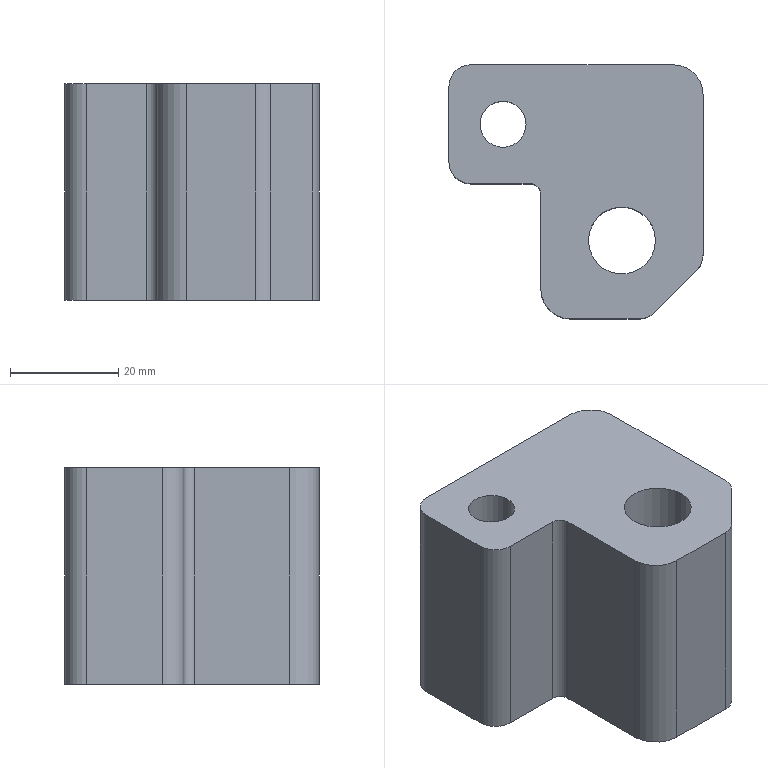Part | NX | features PS-8 2 | 1 solid | 20 faces | box 47 x 47 x 40 mm | volume 60211 mm3 | plane 10 | cylinder 10 | commonest cylinder face diameters 8 x4 11 x2 4 x1 8.5 x1 12.4 x1 14.5 x1
STEP:
#1=CARTESIAN_POINT('',(2465.297,-906.795,860.716));
#2=VERTEX_POINT('',#1);
#3=CARTESIAN_POINT('',(2459.097,-906.795,860.716));
#4=DIRECTION('',(0.,0.,1.));
#5=DIRECTION('',(1.,0.,0.));
#6=AXIS2_PLACEMENT_3D('',#3,#4,#5);
#7=CIRCLE('',#6,6.2);
#8=EDGE_CURVE('',#2,#2,#7,.T.);
#9=ORIENTED_EDGE('',*,*,#8,.T.);
#10=EDGE_LOOP('',(#9));
#11=FACE_BOUND('',#10,.T.);
#12=CARTESIAN_POINT('',(2444.347,-885.295,860.716));
#13=VERTEX_POINT('',#12);
#14=CARTESIAN_POINT('',(2437.097,-885.295,860.716));
#15=DIRECTION('',(0.,0.,1.));
#16=DIRECTION('',(1.,0.,0.));
#17=AXIS2_PLACEMENT_3D('',#14,#15,#16);
#18=CIRCLE('',#17,7.25);
#19=EDGE_CURVE('',#13,#13,#18,.T.);
#20=ORIENTED_EDGE('',*,*,#19,.T.);
#21=EDGE_LOOP('',(#20));
#22=FACE_BOUND('',#21,.T.);
#23=CARTESIAN_POINT('',(2444.097,-898.295,860.716));
#24=VERTEX_POINT('',#23);
#25=CARTESIAN_POINT('',(2444.097,-915.795,860.716));
#26=VERTEX_POINT('',#25);
#27=CARTESIAN_POINT('',(2444.097,0.,860.716));
#28=DIRECTION('',(0.,-1.,0.));
#29=VECTOR('',#28,1000.);
#30=LINE('',#27,#29);
#31=EDGE_CURVE('',#24,#26,#30,.T.);
#32=ORIENTED_EDGE('',*,*,#31,.F.);
#33=CARTESIAN_POINT('',(2442.097,-896.295,860.716));
#34=VERTEX_POINT('',#33);
#35=CARTESIAN_POINT('',(2442.097,-898.295,860.716));
#36=DIRECTION('',(0.,0.,1.));
#37=DIRECTION('',(1.,0.,0.));
#38=AXIS2_PLACEMENT_3D('',#35,#36,#37);
#39=CIRCLE('',#38,2.);
#40=EDGE_CURVE('',#24,#34,#39,.T.);
#41=ORIENTED_EDGE('',*,*,#40,.T.);
#42=CARTESIAN_POINT('',(2431.097,-896.295,860.716));
#43=VERTEX_POINT('',#42);
#44=CARTESIAN_POINT('',(2437.597,-896.295,860.716));
#45=DIRECTION('',(1.,0.,0.));
#46=VECTOR('',#45,1000.);
#47=LINE('',#44,#46);
#48=EDGE_CURVE('',#43,#34,#47,.T.);
#49=ORIENTED_EDGE('',*,*,#48,.F.);
#50=CARTESIAN_POINT('',(2427.097,-892.295,860.716));
#51=VERTEX_POINT('',#50);
#52=CARTESIAN_POINT('',(2431.097,-892.295,860.716));
#53=DIRECTION('',(0.,0.,1.));
#54=DIRECTION('',(1.,0.,0.));
#55=AXIS2_PLACEMENT_3D('',#52,#53,#54);
#56=CIRCLE('',#55,4.);
#57=EDGE_CURVE('',#43,#51,#56,.F.);
#58=ORIENTED_EDGE('',*,*,#57,.T.);
#59=CARTESIAN_POINT('',(2427.097,-878.295,860.716));
#60=VERTEX_POINT('',#59);
#61=CARTESIAN_POINT('',(2427.097,0.,860.716));
#62=DIRECTION('',(0.,-1.,0.));
#63=VECTOR('',#62,1000.);
#64=LINE('',#61,#63);
#65=EDGE_CURVE('',#60,#51,#64,.T.);
#66=ORIENTED_EDGE('',*,*,#65,.F.);
#67=CARTESIAN_POINT('',(2431.097,-874.295,860.716));
#68=VERTEX_POINT('',#67);
#69=CARTESIAN_POINT('',(2431.097,-878.295,860.716));
#70=DIRECTION('',(0.,0.,1.));
#71=DIRECTION('',(1.,0.,0.));
#72=AXIS2_PLACEMENT_3D('',#69,#70,#71);
#73=CIRCLE('',#72,4.);
#74=EDGE_CURVE('',#60,#68,#73,.F.);
#75=ORIENTED_EDGE('',*,*,#74,.T.);
#76=CARTESIAN_POINT('',(2468.597,-874.295,860.716));
#77=VERTEX_POINT('',#76);
#78=CARTESIAN_POINT('',(2468.597,-874.295,860.716));
#79=DIRECTION('',(1.,0.,0.));
#80=VECTOR('',#79,1000.);
#81=LINE('',#78,#80);
#82=EDGE_CURVE('',#68,#77,#81,.T.);
#83=ORIENTED_EDGE('',*,*,#82,.T.);
#84=CARTESIAN_POINT('',(2474.097,-879.795,860.716));
#85=VERTEX_POINT('',#84);
#86=CARTESIAN_POINT('',(2468.597,-879.795,860.716));
#87=DIRECTION('',(0.,0.,1.));
#88=DIRECTION('',(1.,0.,0.));
#89=AXIS2_PLACEMENT_3D('',#86,#87,#88);
#90=CIRCLE('',#89,5.5);
#91=EDGE_CURVE('',#85,#77,#90,.T.);
#92=ORIENTED_EDGE('',*,*,#91,.F.);
#93=CARTESIAN_POINT('',(2474.097,-909.467,860.716));
#94=VERTEX_POINT('',#93);
#95=CARTESIAN_POINT('',(2474.097,0.,860.716));
#96=DIRECTION('',(0.,1.,0.));
#97=VECTOR('',#96,1000.);
#98=LINE('',#95,#97);
#99=EDGE_CURVE('',#94,#85,#98,.T.);
#100=ORIENTED_EDGE('',*,*,#99,.F.);
#101=CARTESIAN_POINT('',(2472.926,-912.295,860.716));
#102=VERTEX_POINT('',#101);
#103=CARTESIAN_POINT('',(2470.097,-909.467,860.716));
#104=DIRECTION('',(0.,0.,1.));
#105=DIRECTION('',(1.,0.,0.));
#106=AXIS2_PLACEMENT_3D('',#103,#104,#105);
#107=CIRCLE('',#106,4.);
#108=EDGE_CURVE('',#94,#102,#107,.F.);
#109=ORIENTED_EDGE('',*,*,#108,.T.);
#110=CARTESIAN_POINT('',(2465.097,-920.124,860.716));
#111=VERTEX_POINT('',#110);
#112=CARTESIAN_POINT('',(1692.61,-1692.61,860.716));
#113=DIRECTION('',(0.7071,0.7071,0.));
#114=VECTOR('',#113,1000.);
#115=LINE('',#112,#114);
#116=EDGE_CURVE('',#111,#102,#115,.T.);
#117=ORIENTED_EDGE('',*,*,#116,.F.);
#118=CARTESIAN_POINT('',(2462.269,-921.295,860.716));
#119=VERTEX_POINT('',#118);
#120=CARTESIAN_POINT('',(2462.269,-917.295,860.716));
#121=DIRECTION('',(0.,0.,1.));
#122=DIRECTION('',(1.,0.,0.));
#123=AXIS2_PLACEMENT_3D('',#120,#121,#122);
#124=CIRCLE('',#123,4.);
#125=EDGE_CURVE('',#119,#111,#124,.T.);
#126=ORIENTED_EDGE('',*,*,#125,.F.);
#127=CARTESIAN_POINT('',(2449.597,-921.295,860.716));
#128=VERTEX_POINT('',#127);
#129=CARTESIAN_POINT('',(2449.597,-921.295,860.716));
#130=DIRECTION('',(-1.,0.,0.));
#131=VECTOR('',#130,1000.);
#132=LINE('',#129,#131);
#133=EDGE_CURVE('',#119,#128,#132,.T.);
#134=ORIENTED_EDGE('',*,*,#133,.T.);
#135=CARTESIAN_POINT('',(2449.597,-915.795,860.716));
#136=DIRECTION('',(0.,0.,1.));
#137=DIRECTION('',(1.,0.,0.));
#138=AXIS2_PLACEMENT_3D('',#135,#136,#137);
#139=CIRCLE('',#138,5.5);
#140=EDGE_CURVE('',#128,#26,#139,.F.);
#141=ORIENTED_EDGE('',*,*,#140,.T.);
#142=EDGE_LOOP('',(#32,#41,#49,#58,#66,#75,#83,#92,#100,#109,#117,#126,#134,#141));
#143=FACE_BOUND('',#142,.T.);
#144=CARTESIAN_POINT('',(0.,0.,860.716));
#145=DIRECTION('',(0.,0.,1.));
#146=DIRECTION('',(1.,0.,0.));
#147=AXIS2_PLACEMENT_3D('',#144,#145,#146);
#148=PLANE('',#147);
#149=ADVANCED_FACE('',(#11,#22,#143),#148,.F.);
#150=CARTESIAN_POINT('',(2444.097,-898.295,900.716));
#151=VERTEX_POINT('',#150);
#152=CARTESIAN_POINT('',(2444.097,-915.795,900.716));
#153=VERTEX_POINT('',#152);
#154=CARTESIAN_POINT('',(2444.097,0.,900.716));
#155=DIRECTION('',(0.,-1.,0.));
#156=VECTOR('',#155,1000.);
#157=LINE('',#154,#156);
#158=EDGE_CURVE('',#151,#153,#157,.T.);
#159=ORIENTED_EDGE('',*,*,#158,.F.);
#160=CARTESIAN_POINT('',(2444.097,-898.295,830.716));
#161=DIRECTION('',(0.,0.,1.));
#162=VECTOR('',#161,1000.);
#163=LINE('',#160,#162);
#164=EDGE_CURVE('',#151,#24,#163,.F.);
#165=ORIENTED_EDGE('',*,*,#164,.T.);
#166=ORIENTED_EDGE('',*,*,#31,.T.);
#167=CARTESIAN_POINT('',(2444.097,-915.795,830.716));
#168=DIRECTION('',(0.,0.,1.));
#169=VECTOR('',#168,1000.);
#170=LINE('',#167,#169);
#171=EDGE_CURVE('',#153,#26,#170,.F.);
#172=ORIENTED_EDGE('',*,*,#171,.F.);
#173=EDGE_LOOP('',(#159,#165,#166,#172));
#174=FACE_BOUND('',#173,.T.);
#175=CARTESIAN_POINT('',(2444.097,-881.795,830.716));
#176=DIRECTION('',(-1.,0.,0.));
#177=DIRECTION('',(0.,0.,1.));
#178=AXIS2_PLACEMENT_3D('',#175,#176,#177);
#179=PLANE('',#178);
#180=ADVANCED_FACE('',(#174),#179,.T.);
#181=ORIENTED_EDGE('',*,*,#171,.T.);
#182=ORIENTED_EDGE('',*,*,#140,.F.);
#183=CARTESIAN_POINT('',(2449.597,-921.295,900.716));
#184=VERTEX_POINT('',#183);
#185=CARTESIAN_POINT('',(2449.597,-921.295,830.716));
#186=DIRECTION('',(0.,0.,-1.));
#187=VECTOR('',#186,1000.);
#188=LINE('',#185,#187);
#189=EDGE_CURVE('',#184,#128,#188,.T.);
#190=ORIENTED_EDGE('',*,*,#189,.F.);
#191=CARTESIAN_POINT('',(2449.597,-915.795,900.716));
#192=DIRECTION('',(0.,0.,1.));
#193=DIRECTION('',(1.,0.,0.));
#194=AXIS2_PLACEMENT_3D('',#191,#192,#193);
#195=CIRCLE('',#194,5.5);
#196=EDGE_CURVE('',#184,#153,#195,.F.);
#197=ORIENTED_EDGE('',*,*,#196,.T.);
#198=EDGE_LOOP('',(#181,#182,#190,#197));
#199=FACE_BOUND('',#198,.T.);
#200=CARTESIAN_POINT('',(2449.597,-915.795,830.716));
#201=DIRECTION('',(0.,0.,1.));
#202=DIRECTION('',(1.,0.,0.));
#203=AXIS2_PLACEMENT_3D('',#200,#201,#202);
#204=CYLINDRICAL_SURFACE('',#203,5.5);
#205=ADVANCED_FACE('',(#199),#204,.T.);
#206=ORIENTED_EDGE('',*,*,#189,.T.);
#207=ORIENTED_EDGE('',*,*,#133,.F.);
#208=CARTESIAN_POINT('',(2462.269,-921.295,900.716));
#209=VERTEX_POINT('',#208);
#210=CARTESIAN_POINT('',(2462.269,-921.295,830.716));
#211=DIRECTION('',(0.,0.,1.));
#212=VECTOR('',#211,1000.);
#213=LINE('',#210,#212);
#214=EDGE_CURVE('',#209,#119,#213,.F.);
#215=ORIENTED_EDGE('',*,*,#214,.F.);
#216=CARTESIAN_POINT('',(0.,-921.295,900.716));
#217=DIRECTION('',(1.,0.,0.));
#218=VECTOR('',#217,1000.);
#219=LINE('',#216,#218);
#220=EDGE_CURVE('',#184,#209,#219,.T.);
#221=ORIENTED_EDGE('',*,*,#220,.F.);
#222=EDGE_LOOP('',(#206,#207,#215,#221));
#223=FACE_BOUND('',#222,.T.);
#224=CARTESIAN_POINT('',(2449.597,-921.295,830.716));
#225=DIRECTION('',(0.,-1.,0.));
#226=DIRECTION('',(0.,0.,-1.));
#227=AXIS2_PLACEMENT_3D('',#224,#225,#226);
#228=PLANE('',#227);
#229=ADVANCED_FACE('',(#223),#228,.T.);
#230=ORIENTED_EDGE('',*,*,#214,.T.);
#231=ORIENTED_EDGE('',*,*,#125,.T.);
#232=CARTESIAN_POINT('',(2465.097,-920.124,900.716));
#233=VERTEX_POINT('',#232);
#234=CARTESIAN_POINT('',(2465.097,-920.124,830.716));
#235=DIRECTION('',(0.,0.,1.));
#236=VECTOR('',#235,1000.);
#237=LINE('',#234,#236);
#238=EDGE_CURVE('',#233,#111,#237,.F.);
#239=ORIENTED_EDGE('',*,*,#238,.F.);
#240=CARTESIAN_POINT('',(2462.269,-917.295,900.716));
#241=DIRECTION('',(0.,0.,1.));
#242=DIRECTION('',(1.,0.,0.));
#243=AXIS2_PLACEMENT_3D('',#240,#241,#242);
#244=CIRCLE('',#243,4.);
#245=EDGE_CURVE('',#209,#233,#244,.T.);
#246=ORIENTED_EDGE('',*,*,#245,.F.);
#247=EDGE_LOOP('',(#230,#231,#239,#246));
#248=FACE_BOUND('',#247,.T.);
#249=CARTESIAN_POINT('',(2462.269,-917.295,830.716));
#250=DIRECTION('',(0.,0.,1.));
#251=DIRECTION('',(1.,0.,0.));
#252=AXIS2_PLACEMENT_3D('',#249,#250,#251);
#253=CYLINDRICAL_SURFACE('',#252,4.);
#254=ADVANCED_FACE('',(#248),#253,.T.);
#255=ORIENTED_EDGE('',*,*,#238,.T.);
#256=ORIENTED_EDGE('',*,*,#116,.T.);
#257=CARTESIAN_POINT('',(2472.926,-912.295,900.716));
#258=VERTEX_POINT('',#257);
#259=CARTESIAN_POINT('',(2472.926,-912.295,830.716));
#260=DIRECTION('',(0.,0.,1.));
#261=VECTOR('',#260,1000.);
#262=LINE('',#259,#261);
#263=EDGE_CURVE('',#258,#102,#262,.F.);
#264=ORIENTED_EDGE('',*,*,#263,.F.);
#265=CARTESIAN_POINT('',(1692.61,-1692.61,900.716));
#266=DIRECTION('',(0.7071,0.7071,0.));
#267=VECTOR('',#266,1000.);
#268=LINE('',#265,#267);
#269=EDGE_CURVE('',#233,#258,#268,.T.);
#270=ORIENTED_EDGE('',*,*,#269,.F.);
#271=EDGE_LOOP('',(#255,#256,#264,#270));
#272=FACE_BOUND('',#271,.T.);
#273=CARTESIAN_POINT('',(2465.097,-920.124,830.716));
#274=DIRECTION('',(0.7071,-0.7071,0.));
#275=DIRECTION('',(0.7071,0.7071,0.));
#276=AXIS2_PLACEMENT_3D('',#273,#274,#275);
#277=PLANE('',#276);
#278=ADVANCED_FACE('',(#272),#277,.T.);
#279=ORIENTED_EDGE('',*,*,#263,.T.);
#280=ORIENTED_EDGE('',*,*,#108,.F.);
#281=CARTESIAN_POINT('',(2474.097,-909.467,900.716));
#282=VERTEX_POINT('',#281);
#283=CARTESIAN_POINT('',(2474.097,-909.467,830.716));
#284=DIRECTION('',(0.,0.,-1.));
#285=VECTOR('',#284,1000.);
#286=LINE('',#283,#285);
#287=EDGE_CURVE('',#282,#94,#286,.T.);
#288=ORIENTED_EDGE('',*,*,#287,.F.);
#289=CARTESIAN_POINT('',(2470.097,-909.467,900.716));
#290=DIRECTION('',(0.,0.,1.));
#291=DIRECTION('',(1.,0.,0.));
#292=AXIS2_PLACEMENT_3D('',#289,#290,#291);
#293=CIRCLE('',#292,4.);
#294=EDGE_CURVE('',#282,#258,#293,.F.);
#295=ORIENTED_EDGE('',*,*,#294,.T.);
#296=EDGE_LOOP('',(#279,#280,#288,#295));
#297=FACE_BOUND('',#296,.T.);
#298=CARTESIAN_POINT('',(2470.097,-909.467,830.716));
#299=DIRECTION('',(0.,0.,1.));
#300=DIRECTION('',(1.,0.,0.));
#301=AXIS2_PLACEMENT_3D('',#298,#299,#300);
#302=CYLINDRICAL_SURFACE('',#301,4.);
#303=ADVANCED_FACE('',(#297),#302,.T.);
#304=ORIENTED_EDGE('',*,*,#287,.T.);
#305=ORIENTED_EDGE('',*,*,#99,.T.);
#306=CARTESIAN_POINT('',(2474.097,-879.795,900.716));
#307=VERTEX_POINT('',#306);
#308=CARTESIAN_POINT('',(2474.097,-879.795,830.716));
#309=DIRECTION('',(0.,0.,1.));
#310=VECTOR('',#309,1000.);
#311=LINE('',#308,#310);
#312=EDGE_CURVE('',#307,#85,#311,.F.);
#313=ORIENTED_EDGE('',*,*,#312,.F.);
#314=CARTESIAN_POINT('',(2474.097,-909.467,900.716));
#315=DIRECTION('',(0.,-1.,0.));
#316=VECTOR('',#315,1000.);
#317=LINE('',#314,#316);
#318=EDGE_CURVE('',#307,#282,#317,.T.);
#319=ORIENTED_EDGE('',*,*,#318,.T.);
#320=EDGE_LOOP('',(#304,#305,#313,#319));
#321=FACE_BOUND('',#320,.T.);
#322=CARTESIAN_POINT('',(2474.097,-909.467,830.716));
#323=DIRECTION('',(1.,0.,0.));
#324=DIRECTION('',(0.,0.,-1.));
#325=AXIS2_PLACEMENT_3D('',#322,#323,#324);
#326=PLANE('',#325);
#327=ADVANCED_FACE('',(#321),#326,.T.);
#328=ORIENTED_EDGE('',*,*,#312,.T.);
#329=ORIENTED_EDGE('',*,*,#91,.T.);
#330=CARTESIAN_POINT('',(2468.597,-874.295,900.716));
#331=VERTEX_POINT('',#330);
#332=CARTESIAN_POINT('',(2468.597,-874.295,830.716));
#333=DIRECTION('',(0.,0.,1.));
#334=VECTOR('',#333,1000.);
#335=LINE('',#332,#334);
#336=EDGE_CURVE('',#331,#77,#335,.F.);
#337=ORIENTED_EDGE('',*,*,#336,.F.);
#338=CARTESIAN_POINT('',(2468.597,-879.795,900.716));
#339=DIRECTION('',(0.,0.,1.));
#340=DIRECTION('',(1.,0.,0.));
#341=AXIS2_PLACEMENT_3D('',#338,#339,#340);
#342=CIRCLE('',#341,5.5);
#343=EDGE_CURVE('',#307,#331,#342,.T.);
#344=ORIENTED_EDGE('',*,*,#343,.F.);
#345=EDGE_LOOP('',(#328,#329,#337,#344));
#346=FACE_BOUND('',#345,.T.);
#347=CARTESIAN_POINT('',(2468.597,-879.795,830.716));
#348=DIRECTION('',(0.,0.,1.));
#349=DIRECTION('',(1.,0.,0.));
#350=AXIS2_PLACEMENT_3D('',#347,#348,#349);
#351=CYLINDRICAL_SURFACE('',#350,5.5);
#352=ADVANCED_FACE('',(#346),#351,.T.);
#353=ORIENTED_EDGE('',*,*,#82,.F.);
#354=CARTESIAN_POINT('',(2431.097,-874.295,900.716));
#355=VERTEX_POINT('',#354);
#356=CARTESIAN_POINT('',(2431.097,-874.295,830.716));
#357=DIRECTION('',(0.,0.,1.));
#358=VECTOR('',#357,1000.);
#359=LINE('',#356,#358);
#360=EDGE_CURVE('',#68,#355,#359,.T.);
#361=ORIENTED_EDGE('',*,*,#360,.T.);
#362=CARTESIAN_POINT('',(2468.597,-874.295,900.716));
#363=DIRECTION('',(1.,0.,0.));
#364=VECTOR('',#363,1000.);
#365=LINE('',#362,#364);
#366=EDGE_CURVE('',#355,#331,#365,.T.);
#367=ORIENTED_EDGE('',*,*,#366,.T.);
#368=ORIENTED_EDGE('',*,*,#336,.T.);
#369=EDGE_LOOP('',(#353,#361,#367,#368));
#370=FACE_BOUND('',#369,.T.);
#371=CARTESIAN_POINT('',(2468.597,-874.295,830.716));
#372=DIRECTION('',(0.,1.,0.));
#373=DIRECTION('',(0.,0.,1.));
#374=AXIS2_PLACEMENT_3D('',#371,#372,#373);
#375=PLANE('',#374);
#376=ADVANCED_FACE('',(#370),#375,.T.);
#377=ORIENTED_EDGE('',*,*,#65,.T.);
#378=CARTESIAN_POINT('',(2427.097,-892.295,900.716));
#379=VERTEX_POINT('',#378);
#380=CARTESIAN_POINT('',(2427.097,-892.295,830.716));
#381=DIRECTION('',(0.,0.,1.));
#382=VECTOR('',#381,1000.);
#383=LINE('',#380,#382);
#384=EDGE_CURVE('',#51,#379,#383,.T.);
#385=ORIENTED_EDGE('',*,*,#384,.T.);
#386=CARTESIAN_POINT('',(2427.097,-878.295,900.716));
#387=VERTEX_POINT('',#386);
#388=CARTESIAN_POINT('',(2427.097,-881.795,900.716));
#389=DIRECTION('',(0.,1.,0.));
#390=VECTOR('',#389,1000.);
#391=LINE('',#388,#390);
#392=EDGE_CURVE('',#379,#387,#391,.T.);
#393=ORIENTED_EDGE('',*,*,#392,.T.);
#394=CARTESIAN_POINT('',(2427.097,-878.295,830.716));
#395=DIRECTION('',(0.,0.,1.));
#396=VECTOR('',#395,1000.);
#397=LINE('',#394,#396);
#398=EDGE_CURVE('',#387,#60,#397,.F.);
#399=ORIENTED_EDGE('',*,*,#398,.T.);
#400=EDGE_LOOP('',(#377,#385,#393,#399));
#401=FACE_BOUND('',#400,.T.);
#402=CARTESIAN_POINT('',(2427.097,-881.795,830.716));
#403=DIRECTION('',(-1.,0.,0.));
#404=DIRECTION('',(0.,0.,1.));
#405=AXIS2_PLACEMENT_3D('',#402,#403,#404);
#406=PLANE('',#405);
#407=ADVANCED_FACE('',(#401),#406,.T.);
#408=ORIENTED_EDGE('',*,*,#48,.T.);
#409=CARTESIAN_POINT('',(2442.097,-896.295,900.716));
#410=VERTEX_POINT('',#409);
#411=CARTESIAN_POINT('',(2442.097,-896.295,875.716));
#412=DIRECTION('',(0.,0.,1.));
#413=VECTOR('',#412,1000.);
#414=LINE('',#411,#413);
#415=EDGE_CURVE('',#34,#410,#414,.T.);
#416=ORIENTED_EDGE('',*,*,#415,.T.);
#417=CARTESIAN_POINT('',(2431.097,-896.295,900.716));
#418=VERTEX_POINT('',#417);
#419=CARTESIAN_POINT('',(2437.597,-896.295,900.716));
#420=DIRECTION('',(1.,0.,0.));
#421=VECTOR('',#420,1000.);
#422=LINE('',#419,#421);
#423=EDGE_CURVE('',#418,#410,#422,.T.);
#424=ORIENTED_EDGE('',*,*,#423,.F.);
#425=CARTESIAN_POINT('',(2431.097,-896.295,875.716));
#426=DIRECTION('',(0.,0.,1.));
#427=VECTOR('',#426,1000.);
#428=LINE('',#425,#427);
#429=EDGE_CURVE('',#418,#43,#428,.F.);
#430=ORIENTED_EDGE('',*,*,#429,.T.);
#431=EDGE_LOOP('',(#408,#416,#424,#430));
#432=FACE_BOUND('',#431,.T.);
#433=CARTESIAN_POINT('',(2437.597,-896.295,875.716));
#434=DIRECTION('',(0.,1.,0.));
#435=DIRECTION('',(0.,0.,1.));
#436=AXIS2_PLACEMENT_3D('',#433,#434,#435);
#437=PLANE('',#436);
#438=ADVANCED_FACE('',(#432),#437,.F.);
#439=CARTESIAN_POINT('',(2442.097,-898.295,900.716));
#440=DIRECTION('',(0.,0.,1.));
#441=DIRECTION('',(1.,0.,0.));
#442=AXIS2_PLACEMENT_3D('',#439,#440,#441);
#443=CIRCLE('',#442,2.);
#444=EDGE_CURVE('',#151,#410,#443,.T.);
#445=ORIENTED_EDGE('',*,*,#444,.T.);
#446=ORIENTED_EDGE('',*,*,#415,.F.);
#447=ORIENTED_EDGE('',*,*,#40,.F.);
#448=ORIENTED_EDGE('',*,*,#164,.F.);
#449=EDGE_LOOP('',(#445,#446,#447,#448));
#450=FACE_BOUND('',#449,.T.);
#451=CARTESIAN_POINT('',(2442.097,-898.295,830.716));
#452=DIRECTION('',(0.,0.,-1.));
#453=DIRECTION('',(-1.,0.,0.));
#454=AXIS2_PLACEMENT_3D('',#451,#452,#453);
#455=CYLINDRICAL_SURFACE('',#454,2.);
#456=ADVANCED_FACE('',(#450),#455,.F.);
#457=CARTESIAN_POINT('',(2431.097,-878.295,900.716));
#458=DIRECTION('',(0.,0.,1.));
#459=DIRECTION('',(1.,0.,0.));
#460=AXIS2_PLACEMENT_3D('',#457,#458,#459);
#461=CIRCLE('',#460,4.);
#462=EDGE_CURVE('',#387,#355,#461,.F.);
#463=ORIENTED_EDGE('',*,*,#462,.T.);
#464=ORIENTED_EDGE('',*,*,#360,.F.);
#465=ORIENTED_EDGE('',*,*,#74,.F.);
#466=ORIENTED_EDGE('',*,*,#398,.F.);
#467=EDGE_LOOP('',(#463,#464,#465,#466));
#468=FACE_BOUND('',#467,.T.);
#469=CARTESIAN_POINT('',(2431.097,-878.295,830.716));
#470=DIRECTION('',(0.,0.,-1.));
#471=DIRECTION('',(-1.,0.,0.));
#472=AXIS2_PLACEMENT_3D('',#469,#470,#471);
#473=CYLINDRICAL_SURFACE('',#472,4.);
#474=ADVANCED_FACE('',(#468),#473,.T.);
#475=CARTESIAN_POINT('',(2431.097,-892.295,900.716));
#476=DIRECTION('',(0.,0.,1.));
#477=DIRECTION('',(1.,0.,0.));
#478=AXIS2_PLACEMENT_3D('',#475,#476,#477);
#479=CIRCLE('',#478,4.);
#480=EDGE_CURVE('',#418,#379,#479,.F.);
#481=ORIENTED_EDGE('',*,*,#480,.T.);
#482=ORIENTED_EDGE('',*,*,#384,.F.);
#483=ORIENTED_EDGE('',*,*,#57,.F.);
#484=ORIENTED_EDGE('',*,*,#429,.F.);
#485=EDGE_LOOP('',(#481,#482,#483,#484));
#486=FACE_BOUND('',#485,.T.);
#487=CARTESIAN_POINT('',(2431.097,-892.295,875.716));
#488=DIRECTION('',(0.,0.,1.));
#489=DIRECTION('',(1.,0.,0.));
#490=AXIS2_PLACEMENT_3D('',#487,#488,#489);
#491=CYLINDRICAL_SURFACE('',#490,4.);
#492=ADVANCED_FACE('',(#486),#491,.T.);
#493=CARTESIAN_POINT('',(2465.297,-906.795,900.716));
#494=VERTEX_POINT('',#493);
#495=CARTESIAN_POINT('',(2459.097,-906.795,900.716));
#496=DIRECTION('',(0.,0.,1.));
#497=DIRECTION('',(1.,0.,0.));
#498=AXIS2_PLACEMENT_3D('',#495,#496,#497);
#499=CIRCLE('',#498,6.2);
#500=EDGE_CURVE('',#494,#494,#499,.F.);
#501=ORIENTED_EDGE('',*,*,#500,.T.);
#502=EDGE_LOOP('',(#501));
#503=FACE_BOUND('',#502,.T.);
#504=CARTESIAN_POINT('',(2441.347,-885.295,900.716));
#505=VERTEX_POINT('',#504);
#506=CARTESIAN_POINT('',(2437.097,-885.295,900.716));
#507=DIRECTION('',(0.,0.,1.));
#508=DIRECTION('',(1.,0.,0.));
#509=AXIS2_PLACEMENT_3D('',#506,#507,#508);
#510=CIRCLE('',#509,4.25);
#511=EDGE_CURVE('',#505,#505,#510,.T.);
#512=ORIENTED_EDGE('',*,*,#511,.F.);
#513=EDGE_LOOP('',(#512));
#514=FACE_BOUND('',#513,.T.);
#515=ORIENTED_EDGE('',*,*,#158,.T.);
#516=ORIENTED_EDGE('',*,*,#196,.F.);
#517=ORIENTED_EDGE('',*,*,#220,.T.);
#518=ORIENTED_EDGE('',*,*,#245,.T.);
#519=ORIENTED_EDGE('',*,*,#269,.T.);
#520=ORIENTED_EDGE('',*,*,#294,.F.);
#521=ORIENTED_EDGE('',*,*,#318,.F.);
#522=ORIENTED_EDGE('',*,*,#343,.T.);
#523=ORIENTED_EDGE('',*,*,#366,.F.);
#524=ORIENTED_EDGE('',*,*,#462,.F.);
#525=ORIENTED_EDGE('',*,*,#392,.F.);
#526=ORIENTED_EDGE('',*,*,#480,.F.);
#527=ORIENTED_EDGE('',*,*,#423,.T.);
#528=ORIENTED_EDGE('',*,*,#444,.F.);
#529=EDGE_LOOP('',(#515,#516,#517,#518,#519,#520,#521,#522,#523,#524,#525,#526,#527,#528));
#530=FACE_BOUND('',#529,.T.);
#531=CARTESIAN_POINT('',(0.,0.,900.716));
#532=DIRECTION('',(0.,0.,1.));
#533=DIRECTION('',(1.,0.,0.));
#534=AXIS2_PLACEMENT_3D('',#531,#532,#533);
#535=PLANE('',#534);
#536=ADVANCED_FACE('',(#503,#514,#530),#535,.T.);
#537=CARTESIAN_POINT('',(2437.097,-878.045,871.716));
#538=VERTEX_POINT('',#537);
#539=CARTESIAN_POINT('',(2437.097,-885.295,871.716));
#540=DIRECTION('',(0.,0.,-1.));
#541=DIRECTION('',(0.,1.,0.));
#542=AXIS2_PLACEMENT_3D('',#539,#540,#541);
#543=CIRCLE('',#542,7.25);
#544=EDGE_CURVE('',#538,#538,#543,.F.);
#545=ORIENTED_EDGE('',*,*,#544,.T.);
#546=EDGE_LOOP('',(#545));
#547=FACE_BOUND('',#546,.T.);
#548=ORIENTED_EDGE('',*,*,#19,.F.);
#549=EDGE_LOOP('',(#548));
#550=FACE_BOUND('',#549,.T.);
#551=CARTESIAN_POINT('',(2437.097,-885.295,871.716));
#552=DIRECTION('',(0.,0.,-1.));
#553=DIRECTION('',(-1.,0.,0.));
#554=AXIS2_PLACEMENT_3D('',#551,#552,#553);
#555=CYLINDRICAL_SURFACE('',#554,7.25);
#556=ADVANCED_FACE('',(#547,#550),#555,.F.);
#557=ORIENTED_EDGE('',*,*,#511,.T.);
#558=EDGE_LOOP('',(#557));
#559=FACE_BOUND('',#558,.T.);
#560=CARTESIAN_POINT('',(2432.847,-885.295,871.716));
#561=VERTEX_POINT('',#560);
#562=CARTESIAN_POINT('',(2437.097,-885.295,871.716));
#563=DIRECTION('',(0.,0.,-1.));
#564=DIRECTION('',(-1.,0.,0.));
#565=AXIS2_PLACEMENT_3D('',#562,#563,#564);
#566=CIRCLE('',#565,4.25);
#567=EDGE_CURVE('',#561,#561,#566,.T.);
#568=ORIENTED_EDGE('',*,*,#567,.T.);
#569=EDGE_LOOP('',(#568));
#570=FACE_BOUND('',#569,.T.);
#571=CARTESIAN_POINT('',(2437.097,-885.295,891.716));
#572=DIRECTION('',(0.,0.,-1.));
#573=DIRECTION('',(-1.,0.,0.));
#574=AXIS2_PLACEMENT_3D('',#571,#572,#573);
#575=CYLINDRICAL_SURFACE('',#574,4.25);
#576=ADVANCED_FACE('',(#559,#570),#575,.F.);
#577=ORIENTED_EDGE('',*,*,#567,.F.);
#578=EDGE_LOOP('',(#577));
#579=FACE_BOUND('',#578,.T.);
#580=ORIENTED_EDGE('',*,*,#544,.F.);
#581=EDGE_LOOP('',(#580));
#582=FACE_BOUND('',#581,.T.);
#583=CARTESIAN_POINT('',(2437.097,-885.295,871.716));
#584=DIRECTION('',(0.,0.,-1.));
#585=DIRECTION('',(-1.,0.,0.));
#586=AXIS2_PLACEMENT_3D('',#583,#584,#585);
#587=PLANE('',#586);
#588=ADVANCED_FACE('',(#579,#582),#587,.T.);
#589=ORIENTED_EDGE('',*,*,#500,.F.);
#590=EDGE_LOOP('',(#589));
#591=FACE_BOUND('',#590,.T.);
#592=ORIENTED_EDGE('',*,*,#8,.F.);
#593=EDGE_LOOP('',(#592));
#594=FACE_BOUND('',#593,.T.);
#595=CARTESIAN_POINT('',(2459.097,-906.795,940.716));
#596=DIRECTION('',(0.,0.,-1.));
#597=DIRECTION('',(-1.,0.,0.));
#598=AXIS2_PLACEMENT_3D('',#595,#596,#597);
#599=CYLINDRICAL_SURFACE('',#598,6.2);
#600=ADVANCED_FACE('',(#591,#594),#599,.F.);
#601=CLOSED_SHELL('',(#149,#180,#205,#229,#254,#278,#303,#327,#352,#376,#407,#438,#456,#474,#492,#536,#556,#576,#588,#600));
#602=MANIFOLD_SOLID_BREP('',#601);
#603=(LENGTH_UNIT()NAMED_UNIT(*)SI_UNIT(.MILLI.,.METRE.));
#604=UNCERTAINTY_MEASURE_WITH_UNIT(LENGTH_MEASURE(0.00001),#603,'','');
#605=(NAMED_UNIT(*)PLANE_ANGLE_UNIT()SI_UNIT($,.RADIAN.));
#606=(NAMED_UNIT(*)SI_UNIT($,.STERADIAN.)SOLID_ANGLE_UNIT());
#607=(GEOMETRIC_REPRESENTATION_CONTEXT(3)GLOBAL_UNCERTAINTY_ASSIGNED_CONTEXT((#604))GLOBAL_UNIT_ASSIGNED_CONTEXT((#603,#605,#606))REPRESENTATION_CONTEXT('',''));
#608=ADVANCED_BREP_SHAPE_REPRESENTATION('',(#602),#607);